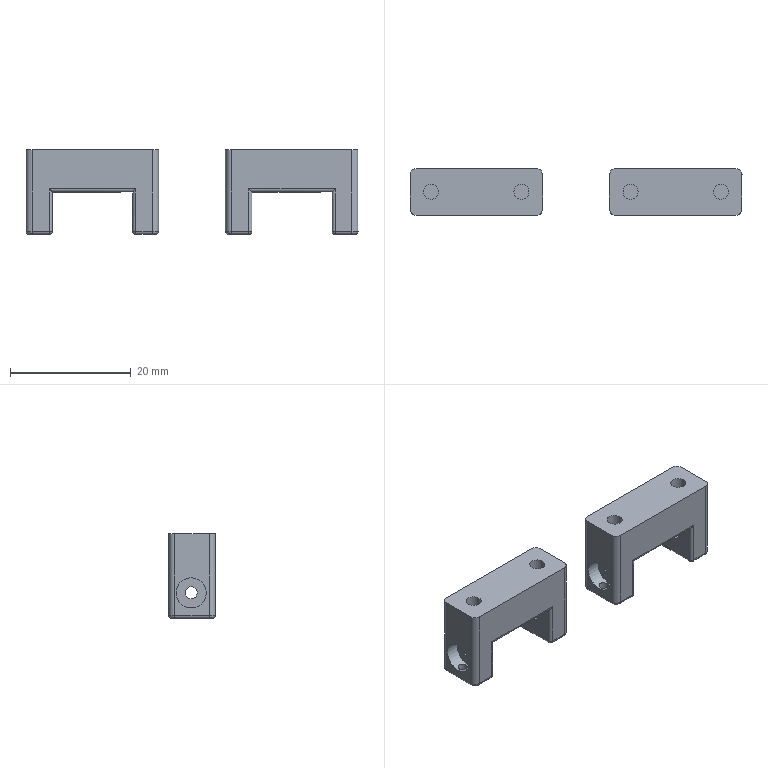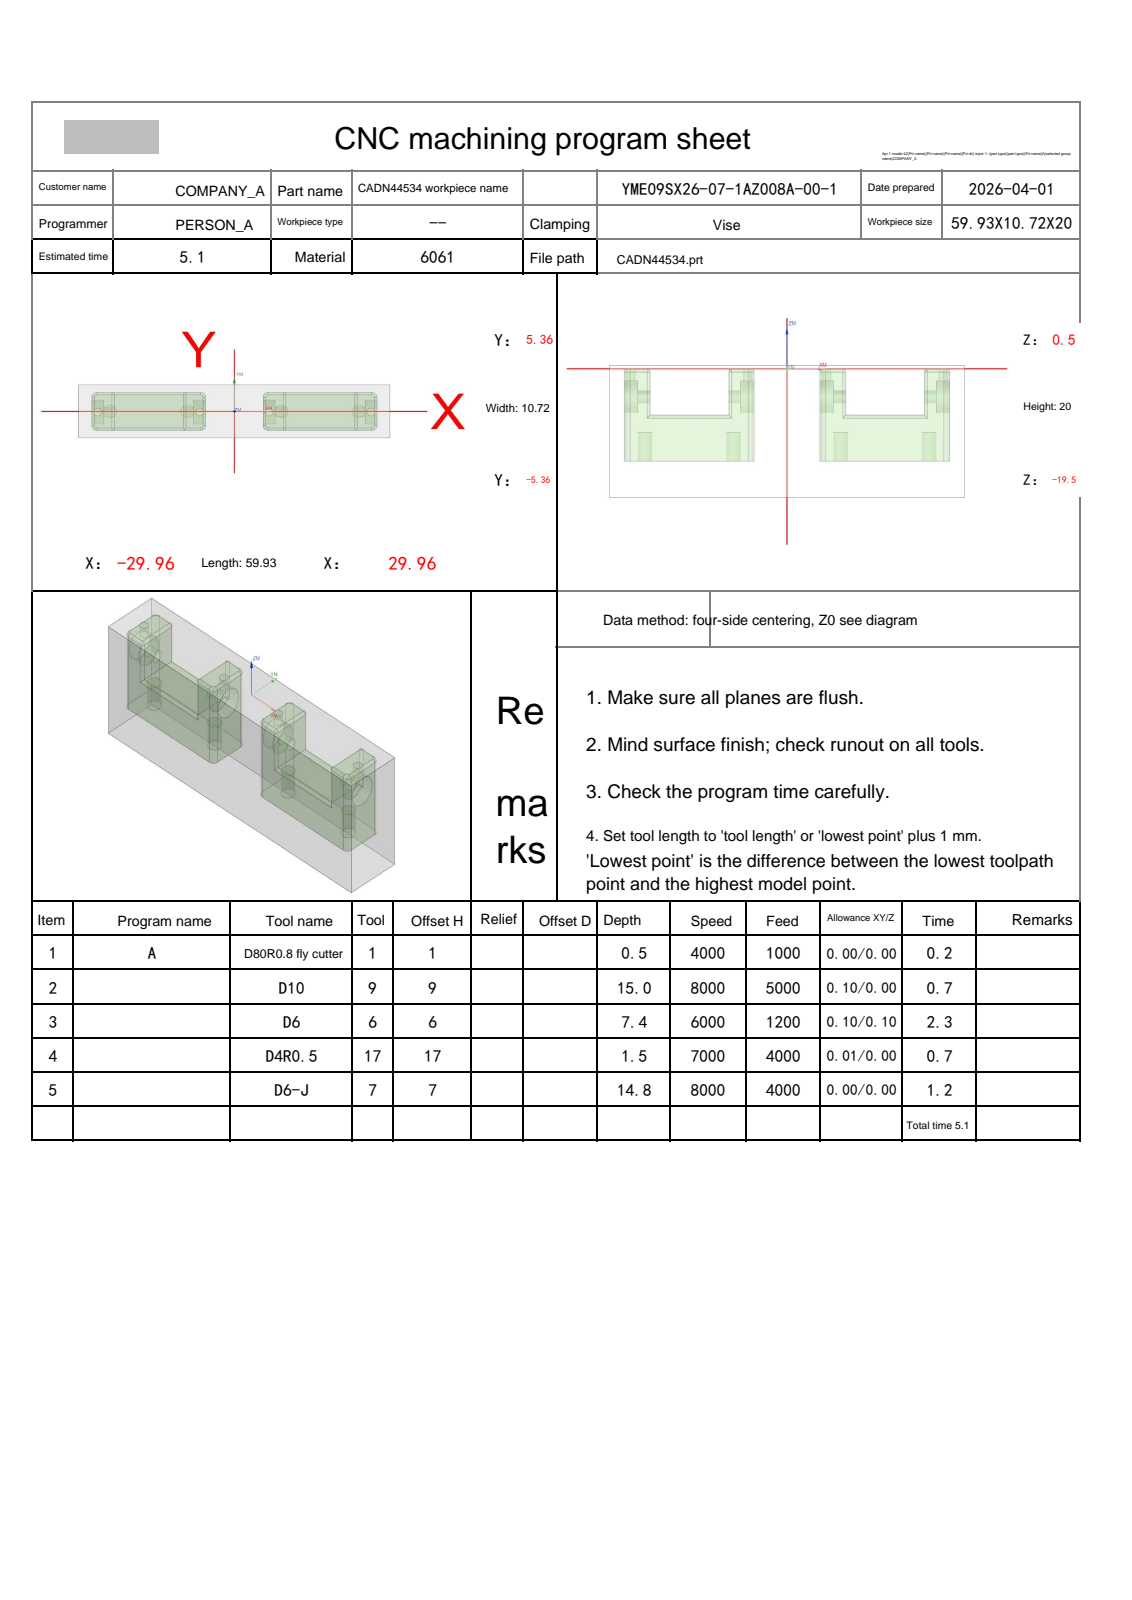NC program | NX | posted by the shop | part box 54.928 x 7.717 x 14 mm
Lines 1 to 1615 of 13497:
%
O0001
(Machine time: 5.96 MIN)
(===Total Tool:5===)
(T1=D80R0.8 fly cutter D=80.  R=0.8  D-  H01 Z=0.    )
(T9=D10     D=10.  R=0.   D-  H09 Z=-14.5 )
(T6=D6      D=6.   R=0.   D-  H06 Z=-6.9  )
(T17=D4R0.5 D=4.   R=0.5  D-  H17 Z=-1.   )
(T7=D6-J    D=6.   R=0.   D7  H07 Z=-14.3 )
G80 G90 G17 G49 G40
G91 G28 Z0
M01
N1 T01 M06
(D80R0.8 fly cutter  D=80. R=0.8 H=01 ce=0.00 di=0.00)
G00 G90 G54 X72.464 Y0.0 M03 S4000
G43 H01 Z20.
M08
Z2.
G01 Z0.0 F1000.
X67.464
X-67.464
X-72.464
Z2.
G00 Z20.
G91 G28 Z0.0
M05
M09
G91 G28 Z0.0
M01
N2 T09 M06
(D10  D=10. R=0. H=09 ce=0.10 di=0.00)
G00 G90 G54 X16.5 Y-8.958 M03 S8000
G43 H09 Z20.
M08
Z0.0
G01 X6.536 Z-.085 F5000.
G02 X.436 Y-2.858 Z-.166 I0.0 J6.1
G01 Y2.858 Z-.215
G02 X6.536 Y8.958 Z-.297 I6.1 J0.0
G01 X26.464 Z-.466
G02 X32.564 Y2.858 Z-.548 I0.0 J-6.1
G01 Y-2.858 Z-.597
G02 X26.464 Y-8.958 Z-.678 I-6.1 J0.0
G01 X6.536 Z-.848
G02 X.436 Y-2.858 Z-.93 I0.0 J6.1
G01 Y2.858 Z-.978
G02 X6.536 Y8.958 Z-1.06 I6.1 J0.0
G01 X26.464 Z-1.23
G02 X32.564 Y2.858 Z-1.311 I0.0 J-6.1
G01 Y-2.858 Z-1.36
G02 X26.464 Y-8.958 Z-1.441 I-6.1 J0.0
G01 X6.536 Z-1.611
G02 X.436 Y-2.858 Z-1.693 I0.0 J6.1
G01 Y2.858 Z-1.741
G02 X6.536 Y8.958 Z-1.823 I6.1 J0.0
G01 X26.464 Z-1.993
G02 X32.564 Y2.858 Z-2.074 I0.0 J-6.1
G01 Y-2.858 Z-2.123
G02 X26.464 Y-8.958 Z-2.205 I-6.1 J0.0
G01 X6.536 Z-2.374
G02 X.436 Y-2.858 Z-2.456 I0.0 J6.1
G01 Y2.858 Z-2.505
G02 X6.536 Y8.958 Z-2.586 I6.1 J0.0
G01 X26.464 Z-2.756
G02 X32.564 Y2.858 Z-2.838 I0.0 J-6.1
G01 Y-2.858 Z-2.886
G02 X26.464 Y-8.958 Z-2.968 I-6.1 J0.0
G01 X6.536 Z-3.138
G02 X.436 Y-2.858 Z-3.219 I0.0 J6.1
G01 Y2.858 Z-3.268
G02 X6.536 Y8.958 Z-3.349 I6.1 J0.0
G01 X26.464 Z-3.519
G02 X32.564 Y2.858 Z-3.601 I0.0 J-6.1
G01 Y-2.858 Z-3.649
G02 X26.464 Y-8.958 Z-3.731 I-6.1 J0.0
G01 X6.536 Z-3.901
G02 X.436 Y-2.858 Z-3.982 I0.0 J6.1
G01 Y2.858 Z-4.031
G02 X6.536 Y8.958 Z-4.113 I6.1 J0.0
G01 X26.464 Z-4.282
G02 X32.564 Y2.858 Z-4.364 I0.0 J-6.1
G01 Y-2.858 Z-4.413
G02 X26.464 Y-8.958 Z-4.494 I-6.1 J0.0
G01 X6.536 Z-4.664
G02 X.436 Y-2.858 Z-4.745 I0.0 J6.1
G01 Y2.858 Z-4.794
G02 X6.536 Y8.958 Z-4.876 I6.1 J0.0
G01 X26.464 Z-5.045
G02 X32.564 Y2.858 Z-5.127 I0.0 J-6.1
G01 Y-2.858 Z-5.176
G02 X26.464 Y-8.958 Z-5.257 I-6.1 J0.0
G01 X6.536 Z-5.427
G02 X.436 Y-2.858 Z-5.509 I0.0 J6.1
G01 Y2.858 Z-5.557
G02 X6.536 Y8.958 Z-5.639 I6.1 J0.0
G01 X26.464 Z-5.809
G02 X32.564 Y2.858 Z-5.89 I0.0 J-6.1
G01 Y-2.858 Z-5.939
G02 X26.464 Y-8.958 Z-6.02 I-6.1 J0.0
G01 X6.536 Z-6.19
G02 X.436 Y-2.858 Z-6.272 I0.0 J6.1
G01 Y2.858 Z-6.32
G02 X6.536 Y8.958 Z-6.402 I6.1 J0.0
G01 X26.464 Z-6.572
G02 X32.564 Y2.858 Z-6.653 I0.0 J-6.1
G01 Y-2.858 Z-6.702
G02 X26.464 Y-8.958 Z-6.784 I-6.1 J0.0
G01 X6.536 Z-6.953
G02 X.436 Y-2.858 Z-7.035 I0.0 J6.1
G01 Y2.858 Z-7.084
G02 X6.536 Y8.958 Z-7.165 I6.1 J0.0
G01 X26.464 Z-7.335
G02 X32.564 Y2.858 Z-7.417 I0.0 J-6.1
G01 Y-2.858 Z-7.465
G02 X26.464 Y-8.958 Z-7.547 I-6.1 J0.0
G01 X6.536 Z-7.716
G02 X.436 Y-2.858 Z-7.798 I0.0 J6.1
G01 Y2.858 Z-7.847
G02 X6.536 Y8.958 Z-7.928 I6.1 J0.0
G01 X26.464 Z-8.098
G02 X32.564 Y2.858 Z-8.18 I0.0 J-6.1
G01 Y-2.858 Z-8.228
G02 X26.464 Y-8.958 Z-8.31 I-6.1 J0.0
G01 X6.536 Z-8.48
G02 X.436 Y-2.858 Z-8.561 I0.0 J6.1
G01 Y2.858 Z-8.61
G02 X6.536 Y8.958 Z-8.692 I6.1 J0.0
G01 X26.464 Z-8.861
G02 X32.564 Y2.858 Z-8.943 I0.0 J-6.1
G01 Y-2.858 Z-8.992
G02 X26.464 Y-8.958 Z-9.073 I-6.1 J0.0
G01 X6.536 Z-9.243
G02 X.436 Y-2.858 Z-9.324 I0.0 J6.1
G01 Y2.858 Z-9.373
G02 X6.536 Y8.958 Z-9.455 I6.1 J0.0
G01 X26.464 Z-9.624
G02 X32.564 Y2.858 Z-9.706 I0.0 J-6.1
G01 Y-2.858 Z-9.755
G02 X26.464 Y-8.958 Z-9.836 I-6.1 J0.0
G01 X6.536 Z-10.006
G02 X.436 Y-2.858 Z-10.088 I0.0 J6.1
G01 Y2.858 Z-10.136
G02 X6.536 Y8.958 Z-10.218 I6.1 J0.0
G01 X26.464 Z-10.388
G02 X32.564 Y2.858 Z-10.469 I0.0 J-6.1
G01 Y-2.858 Z-10.518
G02 X26.464 Y-8.958 Z-10.599 I-6.1 J0.0
G01 X6.536 Z-10.769
G02 X.436 Y-2.858 Z-10.851 I0.0 J6.1
G01 Y2.858 Z-10.899
G02 X6.536 Y8.958 Z-10.981 I6.1 J0.0
G01 X26.464 Z-11.151
G02 X32.564 Y2.858 Z-11.232 I0.0 J-6.1
G01 Y-2.858 Z-11.281
G02 X26.464 Y-8.958 Z-11.363 I-6.1 J0.0
G01 X6.536 Z-11.532
G02 X.436 Y-2.858 Z-11.614 I0.0 J6.1
G01 Y2.858 Z-11.663
G02 X6.536 Y8.958 Z-11.744 I6.1 J0.0
G01 X26.464 Z-11.914
G02 X32.564 Y2.858 Z-11.995 I0.0 J-6.1
G01 Y-2.858 Z-12.044
G02 X26.464 Y-8.958 Z-12.126 I-6.1 J0.0
G01 X6.536 Z-12.295
G02 X.436 Y-2.858 Z-12.377 I0.0 J6.1
G01 Y2.858 Z-12.426
G02 X6.536 Y8.958 Z-12.507 I6.1 J0.0
G01 X26.464 Z-12.677
G02 X32.564 Y2.858 Z-12.759 I0.0 J-6.1
G01 Y-2.858 Z-12.807
G02 X26.464 Y-8.958 Z-12.889 I-6.1 J0.0
G01 X6.536 Z-13.059
G02 X.436 Y-2.858 Z-13.14 I0.0 J6.1
G01 Y2.858 Z-13.189
G02 X6.536 Y8.958 Z-13.271 I6.1 J0.0
G01 X26.464 Z-13.44
G02 X32.564 Y2.858 Z-13.522 I0.0 J-6.1
G01 Y-2.858 Z-13.571
G02 X26.464 Y-8.958 Z-13.652 I-6.1 J0.0
G01 X6.536 Z-13.822
G02 X.436 Y-2.858 Z-13.903 I0.0 J6.1
G01 Y2.858 Z-13.952
G02 X6.536 Y8.958 Z-14.034 I6.1 J0.0
G01 X26.464 Z-14.203
G02 X32.564 Y2.858 Z-14.285 I0.0 J-6.1
G01 Y-2.858 Z-14.334
G02 X26.464 Y-8.958 Z-14.415 I-6.1 J0.0
G01 X16.5 Z-14.5
X6.536
G02 X.436 Y-2.858 I0.0 J6.1
G01 Y2.858
G02 X6.536 Y8.958 I6.1 J0.0
G01 X26.464
G02 X32.564 Y2.858 I0.0 J-6.1
G01 Y-2.858
G02 X26.464 Y-8.958 I-6.1 J0.0
G01 X16.5
X16.
Z-13.5
G00 Z20.
X-16.5
Z0.0
G01 X-26.464 Z-.085
G02 X-32.564 Y-2.858 Z-.166 I0.0 J6.1
G01 Y2.858 Z-.215
G02 X-26.464 Y8.958 Z-.297 I6.1 J0.0
G01 X-6.536 Z-.466
G02 X-.436 Y2.858 Z-.548 I0.0 J-6.1
G01 Y-2.858 Z-.597
G02 X-6.536 Y-8.958 Z-.678 I-6.1 J0.0
G01 X-26.464 Z-.848
G02 X-32.564 Y-2.858 Z-.93 I0.0 J6.1
G01 Y2.858 Z-.978
G02 X-26.464 Y8.958 Z-1.06 I6.1 J0.0
G01 X-6.536 Z-1.23
G02 X-.436 Y2.858 Z-1.311 I0.0 J-6.1
G01 Y-2.858 Z-1.36
G02 X-6.536 Y-8.958 Z-1.441 I-6.1 J0.0
G01 X-26.464 Z-1.611
G02 X-32.564 Y-2.858 Z-1.693 I0.0 J6.1
G01 Y2.858 Z-1.741
G02 X-26.464 Y8.958 Z-1.823 I6.1 J0.0
G01 X-6.536 Z-1.993
G02 X-.436 Y2.858 Z-2.074 I0.0 J-6.1
G01 Y-2.858 Z-2.123
G02 X-6.536 Y-8.958 Z-2.205 I-6.1 J0.0
G01 X-26.464 Z-2.374
G02 X-32.564 Y-2.858 Z-2.456 I0.0 J6.1
G01 Y2.858 Z-2.505
G02 X-26.464 Y8.958 Z-2.586 I6.1 J0.0
G01 X-6.536 Z-2.756
G02 X-.436 Y2.858 Z-2.838 I0.0 J-6.1
G01 Y-2.858 Z-2.886
G02 X-6.536 Y-8.958 Z-2.968 I-6.1 J0.0
G01 X-26.464 Z-3.138
G02 X-32.564 Y-2.858 Z-3.219 I0.0 J6.1
G01 Y2.858 Z-3.268
G02 X-26.464 Y8.958 Z-3.349 I6.1 J0.0
G01 X-6.536 Z-3.519
G02 X-.436 Y2.858 Z-3.601 I0.0 J-6.1
G01 Y-2.858 Z-3.649
G02 X-6.536 Y-8.958 Z-3.731 I-6.1 J0.0
G01 X-26.464 Z-3.901
G02 X-32.564 Y-2.858 Z-3.982 I0.0 J6.1
G01 Y2.858 Z-4.031
G02 X-26.464 Y8.958 Z-4.113 I6.1 J0.0
G01 X-6.536 Z-4.282
G02 X-.436 Y2.858 Z-4.364 I0.0 J-6.1
G01 Y-2.858 Z-4.413
G02 X-6.536 Y-8.958 Z-4.494 I-6.1 J0.0
G01 X-26.464 Z-4.664
G02 X-32.564 Y-2.858 Z-4.745 I0.0 J6.1
G01 Y2.858 Z-4.794
G02 X-26.464 Y8.958 Z-4.876 I6.1 J0.0
G01 X-6.536 Z-5.045
G02 X-.436 Y2.858 Z-5.127 I0.0 J-6.1
G01 Y-2.858 Z-5.176
G02 X-6.536 Y-8.958 Z-5.257 I-6.1 J0.0
G01 X-26.464 Z-5.427
G02 X-32.564 Y-2.858 Z-5.509 I0.0 J6.1
G01 Y2.858 Z-5.557
G02 X-26.464 Y8.958 Z-5.639 I6.1 J0.0
G01 X-6.536 Z-5.809
G02 X-.436 Y2.858 Z-5.89 I0.0 J-6.1
G01 Y-2.858 Z-5.939
G02 X-6.536 Y-8.958 Z-6.02 I-6.1 J0.0
G01 X-26.464 Z-6.19
G02 X-32.564 Y-2.858 Z-6.272 I0.0 J6.1
G01 Y2.858 Z-6.32
G02 X-26.464 Y8.958 Z-6.402 I6.1 J0.0
G01 X-6.536 Z-6.572
G02 X-.436 Y2.858 Z-6.653 I0.0 J-6.1
G01 Y-2.858 Z-6.702
G02 X-6.536 Y-8.958 Z-6.784 I-6.1 J0.0
G01 X-26.464 Z-6.953
G02 X-32.564 Y-2.858 Z-7.035 I0.0 J6.1
G01 Y2.858 Z-7.084
G02 X-26.464 Y8.958 Z-7.165 I6.1 J0.0
G01 X-6.536 Z-7.335
G02 X-.436 Y2.858 Z-7.417 I0.0 J-6.1
G01 Y-2.858 Z-7.465
G02 X-6.536 Y-8.958 Z-7.547 I-6.1 J0.0
G01 X-26.464 Z-7.716
G02 X-32.564 Y-2.858 Z-7.798 I0.0 J6.1
G01 Y2.858 Z-7.847
G02 X-26.464 Y8.958 Z-7.928 I6.1 J0.0
G01 X-6.536 Z-8.098
G02 X-.436 Y2.858 Z-8.18 I0.0 J-6.1
G01 Y-2.858 Z-8.228
G02 X-6.536 Y-8.958 Z-8.31 I-6.1 J0.0
G01 X-26.464 Z-8.48
G02 X-32.564 Y-2.858 Z-8.561 I0.0 J6.1
G01 Y2.858 Z-8.61
G02 X-26.464 Y8.958 Z-8.692 I6.1 J0.0
G01 X-6.536 Z-8.861
G02 X-.436 Y2.858 Z-8.943 I0.0 J-6.1
G01 Y-2.858 Z-8.992
G02 X-6.536 Y-8.958 Z-9.073 I-6.1 J0.0
G01 X-26.464 Z-9.243
G02 X-32.564 Y-2.858 Z-9.324 I0.0 J6.1
G01 Y2.858 Z-9.373
G02 X-26.464 Y8.958 Z-9.455 I6.1 J0.0
G01 X-6.536 Z-9.624
G02 X-.436 Y2.858 Z-9.706 I0.0 J-6.1
G01 Y-2.858 Z-9.755
G02 X-6.536 Y-8.958 Z-9.836 I-6.1 J0.0
G01 X-26.464 Z-10.006
G02 X-32.564 Y-2.858 Z-10.088 I0.0 J6.1
G01 Y2.858 Z-10.136
G02 X-26.464 Y8.958 Z-10.218 I6.1 J0.0
G01 X-6.536 Z-10.388
G02 X-.436 Y2.858 Z-10.469 I0.0 J-6.1
G01 Y-2.858 Z-10.518
G02 X-6.536 Y-8.958 Z-10.599 I-6.1 J0.0
G01 X-26.464 Z-10.769
G02 X-32.564 Y-2.858 Z-10.851 I0.0 J6.1
G01 Y2.858 Z-10.899
G02 X-26.464 Y8.958 Z-10.981 I6.1 J0.0
G01 X-6.536 Z-11.151
G02 X-.436 Y2.858 Z-11.232 I0.0 J-6.1
G01 Y-2.858 Z-11.281
G02 X-6.536 Y-8.958 Z-11.363 I-6.1 J0.0
G01 X-26.464 Z-11.532
G02 X-32.564 Y-2.858 Z-11.614 I0.0 J6.1
G01 Y2.858 Z-11.663
G02 X-26.464 Y8.958 Z-11.744 I6.1 J0.0
G01 X-6.536 Z-11.914
G02 X-.436 Y2.858 Z-11.995 I0.0 J-6.1
G01 Y-2.858 Z-12.044
G02 X-6.536 Y-8.958 Z-12.126 I-6.1 J0.0
G01 X-26.464 Z-12.295
G02 X-32.564 Y-2.858 Z-12.377 I0.0 J6.1
G01 Y2.858 Z-12.426
G02 X-26.464 Y8.958 Z-12.507 I6.1 J0.0
G01 X-6.536 Z-12.677
G02 X-.436 Y2.858 Z-12.759 I0.0 J-6.1
G01 Y-2.858 Z-12.807
G02 X-6.536 Y-8.958 Z-12.889 I-6.1 J0.0
G01 X-26.464 Z-13.059
G02 X-32.564 Y-2.858 Z-13.14 I0.0 J6.1
G01 Y2.858 Z-13.189
G02 X-26.464 Y8.958 Z-13.271 I6.1 J0.0
G01 X-6.536 Z-13.44
G02 X-.436 Y2.858 Z-13.522 I0.0 J-6.1
G01 Y-2.858 Z-13.571
G02 X-6.536 Y-8.958 Z-13.652 I-6.1 J0.0
G01 X-26.464 Z-13.822
G02 X-32.564 Y-2.858 Z-13.903 I0.0 J6.1
G01 Y2.858 Z-13.952
G02 X-26.464 Y8.958 Z-14.034 I6.1 J0.0
G01 X-6.536 Z-14.203
G02 X-.436 Y2.858 Z-14.285 I0.0 J-6.1
G01 Y-2.858 Z-14.334
G02 X-6.536 Y-8.958 Z-14.415 I-6.1 J0.0
G01 X-16.5 Z-14.5
X-26.464
G02 X-32.564 Y-2.858 I0.0 J6.1
G01 Y2.858
G02 X-26.464 Y8.958 I6.1 J0.0
G01 X-6.536
G02 X-.436 Y2.858 I0.0 J-6.1
G01 Y-2.858
G02 X-6.536 Y-8.958 I-6.1 J0.0
G01 X-16.5
X-17.
Z-13.5
G00 Z20.
G91 G28 Z0.0
M05
M09
G91 G28 Z0.0
M01
N3 T06 M06
(D6  D=6. R=0. H=06 ce=0.10 di=0.10)
G00 G90 G54 X16.55 Y9.358 M03 S6000
G43 H06 Z20.
M08
Z.254
G01 Z-.246 F1200.
Y3.958
X20.134
G03 X20.084 Y3.358 I3.55 J-.6
G01 Y-3.358
G03 X20.134 Y-3.958 I3.6 J0.0
G01 X12.966
G03 X13.016 Y-3.358 I-3.55 J.6
G01 Y3.358
G03 X12.966 Y3.958 I-3.6 J0.0
G01 X16.55
Y1.258
X17.384
Y-1.258
X15.716
Y1.258
X16.55
X17.05
Z.254
G00 Z.5
X16.55 Y9.358
Z.008
G01 Z-.492
Y3.958
X20.134
G03 X20.084 Y3.358 I3.55 J-.6
G01 Y-3.358
G03 X20.134 Y-3.958 I3.6 J0.0
G01 X12.966
G03 X13.016 Y-3.358 I-3.55 J.6
G01 Y3.358
G03 X12.966 Y3.958 I-3.6 J0.0
G01 X16.55
Y1.258
X17.384
Y-1.258
X15.716
Y1.258
X16.55
X17.05
Z.008
G00 Z.254
X16.55 Y9.358
Z-.239
G01 Z-.739
Y3.958
X20.134
G03 X20.084 Y3.358 I3.55 J-.6
G01 Y-3.358
G03 X20.134 Y-3.958 I3.6 J0.0
G01 X12.966
G03 X13.016 Y-3.358 I-3.55 J.6
G01 Y3.358
G03 X12.966 Y3.958 I-3.6 J0.0
G01 X16.55
Y1.258
X17.384
Y-1.258
X15.716
Y1.258
X16.55
X17.05
Z-.239
G00 Z.008
X16.55 Y9.358
Z-.485
G01 Z-.985
Y3.958
X20.134
G03 X20.084 Y3.358 I3.55 J-.6
G01 Y-3.358
G03 X20.134 Y-3.958 I3.6 J0.0
G01 X12.966
G03 X13.016 Y-3.358 I-3.55 J.6
G01 Y3.358
G03 X12.966 Y3.958 I-3.6 J0.0
G01 X16.55
Y1.258
X17.384
Y-1.258
X15.716
Y1.258
X16.55
X17.05
Z-.485
G00 Z-.239
X16.55 Y9.358
Z-.732
G01 Z-1.232
Y3.958
X20.134
G03 X20.084 Y3.358 I3.55 J-.6
G01 Y-3.358
G03 X20.134 Y-3.958 I3.6 J0.0
G01 X12.966
G03 X13.016 Y-3.358 I-3.55 J.6
G01 Y3.358
G03 X12.966 Y3.958 I-3.6 J0.0
G01 X16.55
Y1.258
X17.384
Y-1.258
X15.716
Y1.258
X16.55
X17.05
Z-.732
G00 Z-.485
X16.55 Y9.358
Z-.978
G01 Z-1.478
Y3.958
X20.134
G03 X20.084 Y3.358 I3.55 J-.6
G01 Y-3.358
G03 X20.134 Y-3.958 I3.6 J0.0
G01 X12.966
G03 X13.016 Y-3.358 I-3.55 J.6
G01 Y3.358
G03 X12.966 Y3.958 I-3.6 J0.0
G01 X16.55
Y1.258
X17.384
Y-1.258
X15.716
Y1.258
X16.55
X17.05
Z-.978
G00 Z-.732
X16.55 Y9.358
Z-1.225
G01 Z-1.725
Y3.958
X20.134
G03 X20.084 Y3.358 I3.55 J-.6
G01 Y-3.358
G03 X20.134 Y-3.958 I3.6 J0.0
G01 X12.966
G03 X13.016 Y-3.358 I-3.55 J.6
G01 Y3.358
G03 X12.966 Y3.958 I-3.6 J0.0
G01 X16.55
Y1.258
X17.384
Y-1.258
X15.716
Y1.258
X16.55
X17.05
Z-1.225
G00 Z-.978
X16.55 Y9.358
Z-1.471
G01 Z-1.971
Y3.958
X20.134
G03 X20.084 Y3.358 I3.55 J-.6
G01 Y-3.358
G03 X20.134 Y-3.958 I3.6 J0.0
G01 X12.966
G03 X13.016 Y-3.358 I-3.55 J.6
G01 Y3.358
G03 X12.966 Y3.958 I-3.6 J0.0
G01 X16.55
Y1.258
X17.384
Y-1.258
X15.716
Y1.258
X16.55
X17.05
Z-1.471
G00 Z-1.225
X16.55 Y9.358
Z-1.718
G01 Z-2.218
Y3.958
X20.134
G03 X20.084 Y3.358 I3.55 J-.6
G01 Y-3.358
G03 X20.134 Y-3.958 I3.6 J0.0
G01 X12.966
G03 X13.016 Y-3.358 I-3.55 J.6
G01 Y3.358
G03 X12.966 Y3.958 I-3.6 J0.0
G01 X16.55
Y1.258
X17.384
Y-1.258
X15.716
Y1.258
X16.55
X17.05
Z-1.718
G00 Z-1.471
X16.55 Y9.358
Z-1.964
G01 Z-2.464
Y3.958
X20.134
G03 X20.084 Y3.358 I3.55 J-.6
G01 Y-3.358
G03 X20.134 Y-3.958 I3.6 J0.0
G01 X12.966
G03 X13.016 Y-3.358 I-3.55 J.6
G01 Y3.358
G03 X12.966 Y3.958 I-3.6 J0.0
G01 X16.55
Y1.258
X17.384
Y-1.258
X15.716
Y1.258
X16.55
X17.05
Z-1.964
G00 Z-1.718
X16.55 Y9.358
Z-2.21
G01 Z-2.71
Y3.958
X20.134
G03 X20.084 Y3.358 I3.55 J-.6
G01 Y-3.358
G03 X20.134 Y-3.958 I3.6 J0.0
G01 X12.966
G03 X13.016 Y-3.358 I-3.55 J.6
G01 Y3.358
G03 X12.966 Y3.958 I-3.6 J0.0
G01 X16.55
Y1.258
X17.384
Y-1.258
X15.716
Y1.258
X16.55
X17.05
Z-2.21
G00 Z-1.964
X16.55 Y9.358
Z-2.457
G01 Z-2.957
Y3.958
X20.134
G03 X20.084 Y3.358 I3.55 J-.6
G01 Y-3.358
G03 X20.134 Y-3.958 I3.6 J0.0
G01 X12.966
G03 X13.016 Y-3.358 I-3.55 J.6
G01 Y3.358
G03 X12.966 Y3.958 I-3.6 J0.0
G01 X16.55
Y1.258
X17.384
Y-1.258
X15.716
Y1.258
X16.55
X17.05
Z-2.457
G00 Z-2.21
X16.55 Y9.358
Z-2.703
G01 Z-3.203
Y3.958
X20.134
G03 X20.084 Y3.358 I3.55 J-.6
G01 Y-3.358
G03 X20.134 Y-3.958 I3.6 J0.0
G01 X12.966
G03 X13.016 Y-3.358 I-3.55 J.6
G01 Y3.358
G03 X12.966 Y3.958 I-3.6 J0.0
G01 X16.55
Y1.258
X17.384
Y-1.258
X15.716
Y1.258
X16.55
X17.05
Z-2.703
G00 Z-2.457
X16.55 Y9.358
Z-2.95
G01 Z-3.45
Y3.958
X20.134
G03 X20.084 Y3.358 I3.55 J-.6
G01 Y-3.358
G03 X20.134 Y-3.958 I3.6 J0.0
G01 X12.966
G03 X13.016 Y-3.358 I-3.55 J.6
G01 Y3.358
G03 X12.966 Y3.958 I-3.6 J0.0
G01 X16.55
Y1.258
X17.384
Y-1.258
X15.716
Y1.258
X16.55
X17.05
Z-2.95
G00 Z-2.703
X16.55 Y9.358
Z-3.196
G01 Z-3.696
Y3.958
X20.134
G03 X20.084 Y3.358 I3.55 J-.6
G01 Y-3.358
G03 X20.134 Y-3.958 I3.6 J0.0
G01 X12.966
G03 X13.016 Y-3.358 I-3.55 J.6
G01 Y3.358
G03 X12.966 Y3.958 I-3.6 J0.0
G01 X16.55
Y1.258
X17.384
Y-1.258
X15.716
Y1.258
X16.55
X17.05
Z-3.196
G00 Z-2.95
X16.55 Y9.358
Z-3.443
G01 Z-3.943
Y3.958
X20.134
G03 X20.084 Y3.358 I3.55 J-.6
G01 Y-3.358
G03 X20.134 Y-3.958 I3.6 J0.0
G01 X12.966
G03 X13.016 Y-3.358 I-3.55 J.6
G01 Y3.358
G03 X12.966 Y3.958 I-3.6 J0.0
G01 X16.55
Y1.258
X17.384
Y-1.258
X15.716
Y1.258
X16.55
X17.05
Z-3.443
G00 Z-3.196
X16.55 Y9.358
Z-3.689
G01 Z-4.189
Y3.958
X20.134
G03 X20.084 Y3.358 I3.55 J-.6
G01 Y-3.358
G03 X20.134 Y-3.958 I3.6 J0.0
G01 X12.966
G03 X13.016 Y-3.358 I-3.55 J.6
G01 Y3.358
G03 X12.966 Y3.958 I-3.6 J0.0
G01 X16.55
Y1.258
X17.384
Y-1.258
X15.716
Y1.258
X16.55
X17.05
Z-3.689
G00 Z-3.443
X16.55 Y9.358
Z-3.935
G01 Z-4.435
Y3.958
X20.134
G03 X20.084 Y3.358 I3.55 J-.6
G01 Y-3.358
G03 X20.134 Y-3.958 I3.6 J0.0
G01 X12.966
G03 X13.016 Y-3.358 I-3.55 J.6
G01 Y3.358
G03 X12.966 Y3.958 I-3.6 J0.0
G01 X16.55
Y1.258
X17.384
Y-1.258
X15.716
Y1.258
X16.55
X17.05
Z-3.935
G00 Z-3.689
X16.55 Y9.358
Z-4.182
G01 Z-4.682
Y3.958
X20.134
G03 X20.084 Y3.358 I3.55 J-.6
G01 Y-3.358
G03 X20.134 Y-3.958 I3.6 J0.0
G01 X12.966
G03 X13.016 Y-3.358 I-3.55 J.6
G01 Y3.358
G03 X12.966 Y3.958 I-3.6 J0.0
G01 X16.55
Y1.258
X17.384
Y-1.258
X15.716
Y1.258
X16.55
X17.05
Z-4.182
G00 Z-3.935
X16.55 Y9.358
Z-4.428
G01 Z-4.928
Y3.958
X20.134
G03 X20.084 Y3.358 I3.55 J-.6
G01 Y-3.358
G03 X20.134 Y-3.958 I3.6 J0.0
G01 X12.966
G03 X13.016 Y-3.358 I-3.55 J.6
G01 Y3.358
G03 X12.966 Y3.958 I-3.6 J0.0
G01 X16.55
Y1.258
X17.384
Y-1.258
X15.716
Y1.258
X16.55
X17.05
Z-4.428
G00 Z-4.182
X16.55 Y9.358
Z-4.675
G01 Z-5.175
Y3.958
X20.134
G03 X20.084 Y3.358 I3.55 J-.6
G01 Y-3.358
G03 X20.134 Y-3.958 I3.6 J0.0
G01 X12.966
G03 X13.016 Y-3.358 I-3.55 J.6
G01 Y3.358
G03 X12.966 Y3.958 I-3.6 J0.0
G01 X16.55
Y1.258
X17.384
Y-1.258
X15.716
Y1.258
X16.55
X17.05
Z-4.675
G00 Z-4.428
X16.55 Y9.358
Z-4.921
G01 Z-5.421
Y3.958
X20.134
G03 X20.084 Y3.358 I3.55 J-.6
G01 Y-3.358
G03 X20.134 Y-3.958 I3.6 J0.0
G01 X12.966
G03 X13.016 Y-3.358 I-3.55 J.6
G01 Y3.358
G03 X12.966 Y3.958 I-3.6 J0.0
G01 X16.55
Y1.258
X17.384
Y-1.258
X15.716
Y1.258
X16.55
X17.05
Z-4.921
G00 Z-4.675
X16.55 Y9.358
Z-5.168
G01 Z-5.668
Y3.958
X20.134
G03 X20.084 Y3.358 I3.55 J-.6
G01 Y-3.358
G03 X20.134 Y-3.958 I3.6 J0.0
G01 X12.966
G03 X13.016 Y-3.358 I-3.55 J.6
G01 Y3.358
G03 X12.966 Y3.958 I-3.6 J0.0
G01 X16.55
Y1.258
X17.384
Y-1.258
X15.716
Y1.258
X16.55
X17.05
Z-5.168
G00 Z-4.921
X16.55 Y9.358
Z-5.414
G01 Z-5.914
Y3.958
X20.134
G03 X20.084 Y3.358 I3.55 J-.6
G01 Y-3.358
G03 X20.134 Y-3.958 I3.6 J0.0
G01 X12.966
G03 X13.016 Y-3.358 I-3.55 J.6
G01 Y3.358
G03 X12.966 Y3.958 I-3.6 J0.0
G01 X16.55
Y1.258
X17.384
Y-1.258
X15.716
Y1.258
X16.55
X17.05
Z-5.414
G00 Z-5.168
X16.55 Y9.358
Z-5.66
G01 Z-6.16
Y3.958
X20.134
G03 X20.084 Y3.358 I3.55 J-.6
G01 Y-3.358
G03 X20.134 Y-3.958 I3.6 J0.0
G01 X12.966
G03 X13.016 Y-3.358 I-3.55 J.6
G01 Y3.358
G03 X12.966 Y3.958 I-3.6 J0.0
G01 X16.55
Y1.258
X17.384
Y-1.258
X15.716
Y1.258
X16.55
X17.05
Z-5.66
G00 Z-5.414
X16.55 Y9.358
Z-5.907
G01 Z-6.407
Y3.958
X20.134
G03 X20.084 Y3.358 I3.55 J-.6
G01 Y-3.358
G03 X20.134 Y-3.958 I3.6 J0.0
G01 X12.966
G03 X13.016 Y-3.358 I-3.55 J.6
G01 Y3.358
G03 X12.966 Y3.958 I-3.6 J0.0
G01 X16.55
Y1.258
X17.384
Y-1.258
X15.716
Y1.258
X16.55
X17.05
Z-5.907
G00 Z-5.66
X16.55 Y9.358
Z-6.153
G01 Z-6.653
Y3.958
X20.134
G03 X20.084 Y3.358 I3.55 J-.6
G01 Y-3.358
G03 X20.134 Y-3.958 I3.6 J0.0
G01 X12.966
G03 X13.016 Y-3.358 I-3.55 J.6
G01 Y3.358
G03 X12.966 Y3.958 I-3.6 J0.0
G01 X16.55
Y1.258
X17.384
Y-1.258
X15.716
Y1.258
X16.55
X17.05
Z-6.153
G00 Z-5.907
X16.55 Y9.358
Z-6.4
G01 Z-6.9
Y3.958
X20.134
G03 X20.084 Y3.358 I3.55 J-.6
G01 Y-3.358
G03 X20.134 Y-3.958 I3.6 J0.0
G01 X12.966
G03 X13.016 Y-3.358 I-3.55 J.6
G01 Y3.358
G03 X12.966 Y3.958 I-3.6 J0.0
G01 X16.55
Y1.258
X17.384
Y-1.258
X15.716
Y1.258
X16.55
X17.05
Z-6.4
G00 Z20.
X-16.45 Y9.358
Z.254
G01 Z-.246
Y3.958
X-12.866
G03 X-12.916 Y3.358 I3.55 J-.6
G01 Y-3.358
G03 X-12.866 Y-3.958 I3.6 J0.0
G01 X-20.034
G03 X-19.984 Y-3.358 I-3.55 J.6
G01 Y3.358
G03 X-20.034 Y3.958 I-3.6 J0.0
G01 X-16.45
Y1.258
X-15.616
Y-1.258
X-17.284
Y1.258
X-16.45
X-15.95
Z.254
G00 Z.5
X-16.45 Y9.358
Z.007
G01 Z-.493
Y3.958
X-12.866
G03 X-12.916 Y3.358 I3.55 J-.6
G01 Y-3.358
G03 X-12.866 Y-3.958 I3.6 J0.0
G01 X-20.034
G03 X-19.984 Y-3.358 I-3.55 J.6
G01 Y3.358
G03 X-20.034 Y3.958 I-3.6 J0.0
G01 X-16.45
Y1.258
X-15.616
Y-1.258
X-17.284
Y1.258
X-16.45
X-15.95
Z.007
G00 Z.254
X-16.45 Y9.358
Z-.239
G01 Z-.739
Y3.958
X-12.866
G03 X-12.916 Y3.358 I3.55 J-.6
G01 Y-3.358
G03 X-12.866 Y-3.958 I3.6 J0.0
G01 X-20.034
G03 X-19.984 Y-3.358 I-3.55 J.6
G01 Y3.358
G03 X-20.034 Y3.958 I-3.6 J0.0
G01 X-16.45
Y1.258
X-15.616
Y-1.258
X-17.284
Y1.258
X-16.45
X-15.95
Z-.239
G00 Z.007
X-16.45 Y9.358
Z-.485
G01 Z-.985
Y3.958
X-12.866
G03 X-12.916 Y3.358 I3.55 J-.6
G01 Y-3.358
G03 X-12.866 Y-3.958 I3.6 J0.0
G01 X-20.034
G03 X-19.984 Y-3.358 I-3.55 J.6
G01 Y3.358
G03 X-20.034 Y3.958 I-3.6 J0.0
G01 X-16.45
Y1.258
X-15.616
Y-1.258
X-17.284
Y1.258
X-16.45
X-15.95
Z-.485
G00 Z-.239
X-16.45 Y9.358
Z-.732
G01 Z-1.232
Y3.958
X-12.866
G03 X-12.916 Y3.358 I3.55 J-.6
G01 Y-3.358
G03 X-12.866 Y-3.958 I3.6 J0.0
G01 X-20.034
G03 X-19.984 Y-3.358 I-3.55 J.6
G01 Y3.358
G03 X-20.034 Y3.958 I-3.6 J0.0
G01 X-16.45
Y1.258
X-15.616
Y-1.258
X-17.284
Y1.258
X-16.45
X-15.95
Z-.732
G00 Z-.485
X-16.45 Y9.358
Z-.978
G01 Z-1.478
Y3.958
X-12.866
G03 X-12.916 Y3.358 I3.55 J-.6
G01 Y-3.358
G03 X-12.866 Y-3.958 I3.6 J0.0
G01 X-20.034
G03 X-19.984 Y-3.358 I-3.55 J.6
G01 Y3.358
G03 X-20.034 Y3.958 I-3.6 J0.0
G01 X-16.45
Y1.258
X-15.616
Y-1.258
X-17.284
Y1.258
X-16.45
X-15.95
Z-.978
G00 Z-.732
X-16.45 Y9.358
Z-1.225
G01 Z-1.725
Y3.958
X-12.866
G03 X-12.916 Y3.358 I3.55 J-.6
G01 Y-3.358
G03 X-12.866 Y-3.958 I3.6 J0.0
G01 X-20.034
G03 X-19.984 Y-3.358 I-3.55 J.6
G01 Y3.358
G03 X-20.034 Y3.958 I-3.6 J0.0
G01 X-16.45
Y1.258
X-15.616
Y-1.258
X-17.284
Y1.258
X-16.45
X-15.95
Z-1.225
G00 Z-.978
X-16.45 Y9.358
Z-1.471
G01 Z-1.971
Y3.958
X-12.866
G03 X-12.916 Y3.358 I3.55 J-.6
G01 Y-3.358
G03 X-12.866 Y-3.958 I3.6 J0.0
G01 X-20.034
G03 X-19.984 Y-3.358 I-3.55 J.6
G01 Y3.358
G03 X-20.034 Y3.958 I-3.6 J0.0
G01 X-16.45
Y1.258
X-15.616
Y-1.258
X-17.284
Y1.258
X-16.45
X-15.95
Z-1.471
G00 Z-1.225
X-16.45 Y9.358
Z-1.718
G01 Z-2.218
Y3.958
X-12.866
G03 X-12.916 Y3.358 I3.55 J-.6
G01 Y-3.358
G03 X-12.866 Y-3.958 I3.6 J0.0
G01 X-20.034
G03 X-19.984 Y-3.358 I-3.55 J.6
G01 Y3.358
G03 X-20.034 Y3.958 I-3.6 J0.0
G01 X-16.45
Y1.258
X-15.616
Y-1.258
X-17.284
Y1.258
X-16.45
X-15.95
Z-1.718
G00 Z-1.471
X-16.45 Y9.358
Z-1.964
G01 Z-2.464
Y3.958
X-12.866
G03 X-12.916 Y3.358 I3.55 J-.6
G01 Y-3.358
G03 X-12.866 Y-3.958 I3.6 J0.0
G01 X-20.034
G03 X-19.984 Y-3.358 I-3.55 J.6
G01 Y3.358
G03 X-20.034 Y3.958 I-3.6 J0.0
G01 X-16.45
Y1.258
X-15.616
Y-1.258
X-17.284
Y1.258
X-16.45
X-15.95
Z-1.964
G00 Z-1.718
X-16.45 Y9.358
Z-2.211
G01 Z-2.711
Y3.958
X-12.866
G03 X-12.916 Y3.358 I3.55 J-.6
G01 Y-3.358
G03 X-12.866 Y-3.958 I3.6 J0.0
G01 X-20.034
G03 X-19.984 Y-3.358 I-3.55 J.6
G01 Y3.358
G03 X-20.034 Y3.958 I-3.6 J0.0
G01 X-16.45
Y1.258
X-15.616
Y-1.258
X-17.284
Y1.258
X-16.45
X-15.95
Z-2.211
G00 Z-1.964
X-16.45 Y9.358
Z-2.457
G01 Z-2.957
Y3.958
X-12.866
G03 X-12.916 Y3.358 I3.55 J-.6
G01 Y-3.358
G03 X-12.866 Y-3.958 I3.6 J0.0
G01 X-20.034
G03 X-19.984 Y-3.358 I-3.55 J.6
G01 Y3.358
G03 X-20.034 Y3.958 I-3.6 J0.0
G01 X-16.45
Y1.258
X-15.616
Y-1.258
X-17.284
Y1.258
X-16.45
X-15.95
Z-2.457
G00 Z-2.211
X-16.45 Y9.358
Z-2.703
G01 Z-3.203
Y3.958
X-12.866
G03 X-12.916 Y3.358 I3.55 J-.6
G01 Y-3.358
G03 X-12.866 Y-3.958 I3.6 J0.0
G01 X-20.034
G03 X-19.984 Y-3.358 I-3.55 J.6
G01 Y3.358
G03 X-20.034 Y3.958 I-3.6 J0.0
G01 X-16.45
Y1.258
X-15.616
Y-1.258
X-17.284
Y1.258
X-16.45
X-15.95
Z-2.703
G00 Z-2.457
X-16.45 Y9.358
Z-2.95
G01 Z-3.45
Y3.958
X-12.866
G03 X-12.916 Y3.358 I3.55 J-.6
G01 Y-3.358
G03 X-12.866 Y-3.958 I3.6 J0.0
G01 X-20.034
G03 X-19.984 Y-3.358 I-3.55 J.6
G01 Y3.358
G03 X-20.034 Y3.958 I-3.6 J0.0
G01 X-16.45
Y1.258
X-15.616
Y-1.258
X-17.284
Y1.258
X-16.45
X-15.95
Z-2.95
G00 Z-2.703
X-16.45 Y9.358
Z-3.196
G01 Z-3.696
Y3.958
X-12.866
G03 X-12.916 Y3.358 I3.55 J-.6
G01 Y-3.358
G03 X-12.866 Y-3.958 I3.6 J0.0
G01 X-20.034
G03 X-19.984 Y-3.358 I-3.55 J.6
G01 Y3.358
G03 X-20.034 Y3.958 I-3.6 J0.0
G01 X-16.45
Y1.258
X-15.616
Y-1.258
X-17.284
Y1.258
X-16.45
X-15.95
Z-3.196
G00 Z-2.95
X-16.45 Y9.358
Z-3.443
G01 Z-3.943
Y3.958
X-12.866
G03 X-12.916 Y3.358 I3.55 J-.6
G01 Y-3.358
G03 X-12.866 Y-3.958 I3.6 J0.0
G01 X-20.034
G03 X-19.984 Y-3.358 I-3.55 J.6
G01 Y3.358
G03 X-20.034 Y3.958 I-3.6 J0.0
G01 X-16.45
Y1.258
X-15.616
Y-1.258
X-17.284
Y1.258
X-16.45
X-15.95
Z-3.443
G00 Z-3.196
X-16.45 Y9.358
Z-3.689
G01 Z-4.189
Y3.958
X-12.866
G03 X-12.916 Y3.358 I3.55 J-.6
G01 Y-3.358
G03 X-12.866 Y-3.958 I3.6 J0.0
G01 X-20.034
G03 X-19.984 Y-3.358 I-3.55 J.6
G01 Y3.358
G03 X-20.034 Y3.958 I-3.6 J0.0
G01 X-16.45
Y1.258
X-15.616
Y-1.258
X-17.284
Y1.258
X-16.45
X-15.95
Z-3.689
G00 Z-3.443
X-16.45 Y9.358
Z-3.936
G01 Z-4.436
Y3.958
X-12.866
G03 X-12.916 Y3.358 I3.55 J-.6
G01 Y-3.358
G03 X-12.866 Y-3.958 I3.6 J0.0
G01 X-20.034
G03 X-19.984 Y-3.358 I-3.55 J.6
G01 Y3.358
G03 X-20.034 Y3.958 I-3.6 J0.0
G01 X-16.45
Y1.258
X-15.616
Y-1.258
X-17.284
Y1.258
X-16.45
X-15.95
Z-3.936
G00 Z-3.689
X-16.45 Y9.358
Z-4.182
G01 Z-4.682
Y3.958
X-12.866
G03 X-12.916 Y3.358 I3.55 J-.6
G01 Y-3.358
G03 X-12.866 Y-3.958 I3.6 J0.0
G01 X-20.034
G03 X-19.984 Y-3.358 I-3.55 J.6
G01 Y3.358
G03 X-20.034 Y3.958 I-3.6 J0.0
G01 X-16.45
Y1.258
X-15.616
Y-1.258
X-17.284
Y1.258
X-16.45
X-15.95
Z-4.182
G00 Z-3.936
X-16.45 Y9.358
Z-4.428
G01 Z-4.928
Y3.958
X-12.866
G03 X-12.916 Y3.358 I3.55 J-.6
G01 Y-3.358
G03 X-12.866 Y-3.958 I3.6 J0.0
G01 X-20.034
G03 X-19.984 Y-3.358 I-3.55 J.6
G01 Y3.358
G03 X-20.034 Y3.958 I-3.6 J0.0
G01 X-16.45
Y1.258
X-15.616
Y-1.258
X-17.284
Y1.258
X-16.45
X-15.95
Z-4.428
G00 Z-4.182
X-16.45 Y9.358
Z-4.675
G01 Z-5.175
Y3.958
X-12.866
G03 X-12.916 Y3.358 I3.55 J-.6
G01 Y-3.358
G03 X-12.866 Y-3.958 I3.6 J0.0
G01 X-20.034
G03 X-19.984 Y-3.358 I-3.55 J.6
G01 Y3.358
G03 X-20.034 Y3.958 I-3.6 J0.0
G01 X-16.45
Y1.258
X-15.616
Y-1.258
X-17.284
Y1.258
X-16.45
X-15.95
Z-4.675
G00 Z-4.428
X-16.45 Y9.358
Z-4.921
G01 Z-5.421
Y3.958
X-12.866
G03 X-12.916 Y3.358 I3.55 J-.6
G01 Y-3.358
G03 X-12.866 Y-3.958 I3.6 J0.0
G01 X-20.034
G03 X-19.984 Y-3.358 I-3.55 J.6
G01 Y3.358
G03 X-20.034 Y3.958 I-3.6 J0.0
G01 X-16.45
Y1.258
X-15.616
Y-1.258
X-17.284
Y1.258
X-16.45
X-15.95
Z-4.921
G00 Z-4.675
X-16.45 Y9.358
Z-5.168
G01 Z-5.668
Y3.958
X-12.866
G03 X-12.916 Y3.358 I3.55 J-.6
G01 Y-3.358
G03 X-12.866 Y-3.958 I3.6 J0.0
G01 X-20.034
G03 X-19.984 Y-3.358 I-3.55 J.6
G01 Y3.358
G03 X-20.034 Y3.958 I-3.6 J0.0
G01 X-16.45
Y1.258
X-15.616
Y-1.258
X-17.284
Y1.258
X-16.45
X-15.95
Z-5.168
G00 Z-4.921
X-16.45 Y9.358
Z-5.414
G01 Z-5.914
Y3.958
X-12.866
G03 X-12.916 Y3.358 I3.55 J-.6
G01 Y-3.358
G03 X-12.866 Y-3.958 I3.6 J0.0
G01 X-20.034
G03 X-19.984 Y-3.358 I-3.55 J.6
G01 Y3.358
G03 X-20.034 Y3.958 I-3.6 J0.0
G01 X-16.45
Y1.258
X-15.616
Y-1.258
X-17.284
Y1.258
X-16.45
X-15.95
Z-5.414
G00 Z-5.168
X-16.45 Y9.358
Z-5.661
G01 Z-6.161
Y3.958
X-12.866
G03 X-12.916 Y3.358 I3.55 J-.6
G01 Y-3.358
G03 X-12.866 Y-3.958 I3.6 J0.0
G01 X-20.034
G03 X-19.984 Y-3.358 I-3.55 J.6
G01 Y3.358
G03 X-20.034 Y3.958 I-3.6 J0.0
G01 X-16.45
Y1.258
X-15.616
Y-1.258
X-17.284
Y1.258
X-16.45
X-15.95
Z-5.661
G00 Z-5.414
X-16.45 Y9.358
Z-5.907
G01 Z-6.407
Y3.958
X-12.866
G03 X-12.916 Y3.358 I3.55 J-.6
G01 Y-3.358
G03 X-12.866 Y-3.958 I3.6 J0.0
G01 X-20.034
G03 X-19.984 Y-3.358 I-3.55 J.6
G01 Y3.358
G03 X-20.034 Y3.958 I-3.6 J0.0
G01 X-16.45
Y1.258
X-15.616
Y-1.258
X-17.284
Y1.258
X-16.45
X-15.95
Z-5.907
G00 Z-5.661
X-16.45 Y9.358
Z-6.153
G01 Z-6.653
Y3.958
X-12.866
G03 X-12.916 Y3.358 I3.55 J-.6
G01 Y-3.358
G03 X-12.866 Y-3.958 I3.6 J0.0
G01 X-20.034
G03 X-19.984 Y-3.358 I-3.55 J.6
G01 Y3.358
G03 X-20.034 Y3.958 I-3.6 J0.0
G01 X-16.45
Y1.258
X-15.616
Y-1.258
X-17.284
Y1.258
X-16.45
X-15.95
Z-6.153
G00 Z-5.907
X-16.45 Y9.358
Z-6.4
G01 Z-6.9
Y3.958
X-12.866
G03 X-12.916 Y3.358 I3.55 J-.6
G01 Y-3.358
G03 X-12.866 Y-3.958 I3.6 J0.0
G01 X-20.034
G03 X-19.984 Y-3.358 I-3.55 J.6
G01 Y3.358
G03 X-20.034 Y3.958 I-3.6 J0.0
G01 X-16.45
Y1.258
X-15.616
Y-1.258
X-17.284
Y1.258
X-16.45
X-15.95
Z-6.4
G00 Z20.
G91 G28 Z0.0
M05
M09
G91 G28 Z0.0
M01